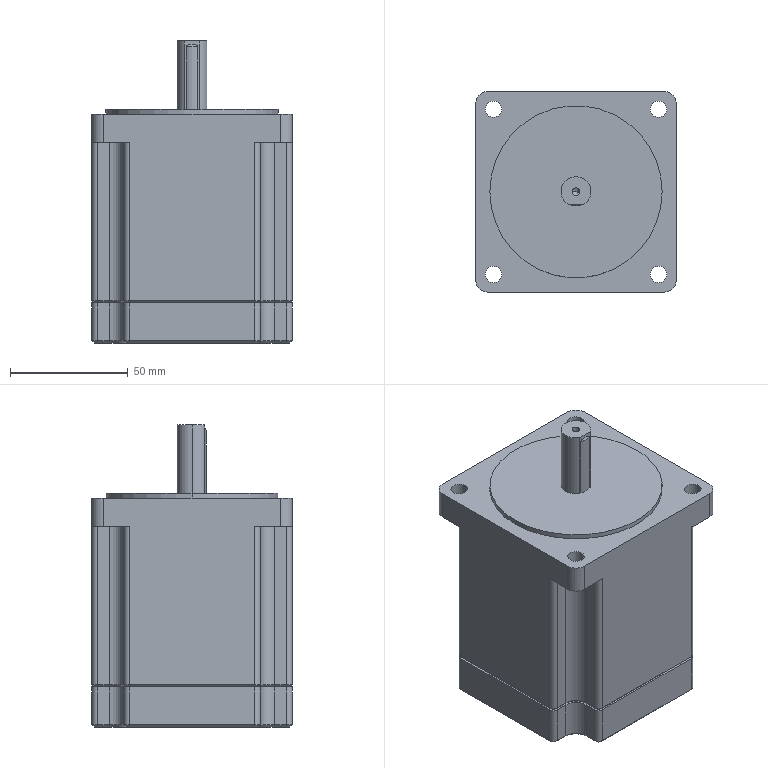Part | STEP file | BS86HB80-04 | 1 solid | 129 faces | box 85 x 85 x 128 mm | volume 650042 mm3 | plane 58 | cylinder 44 | cone 26 | spline 1 | commonest cylinder face diameters 5 x16 12 x9 7 x8 10 x4 12.7 x3 3.3 x2